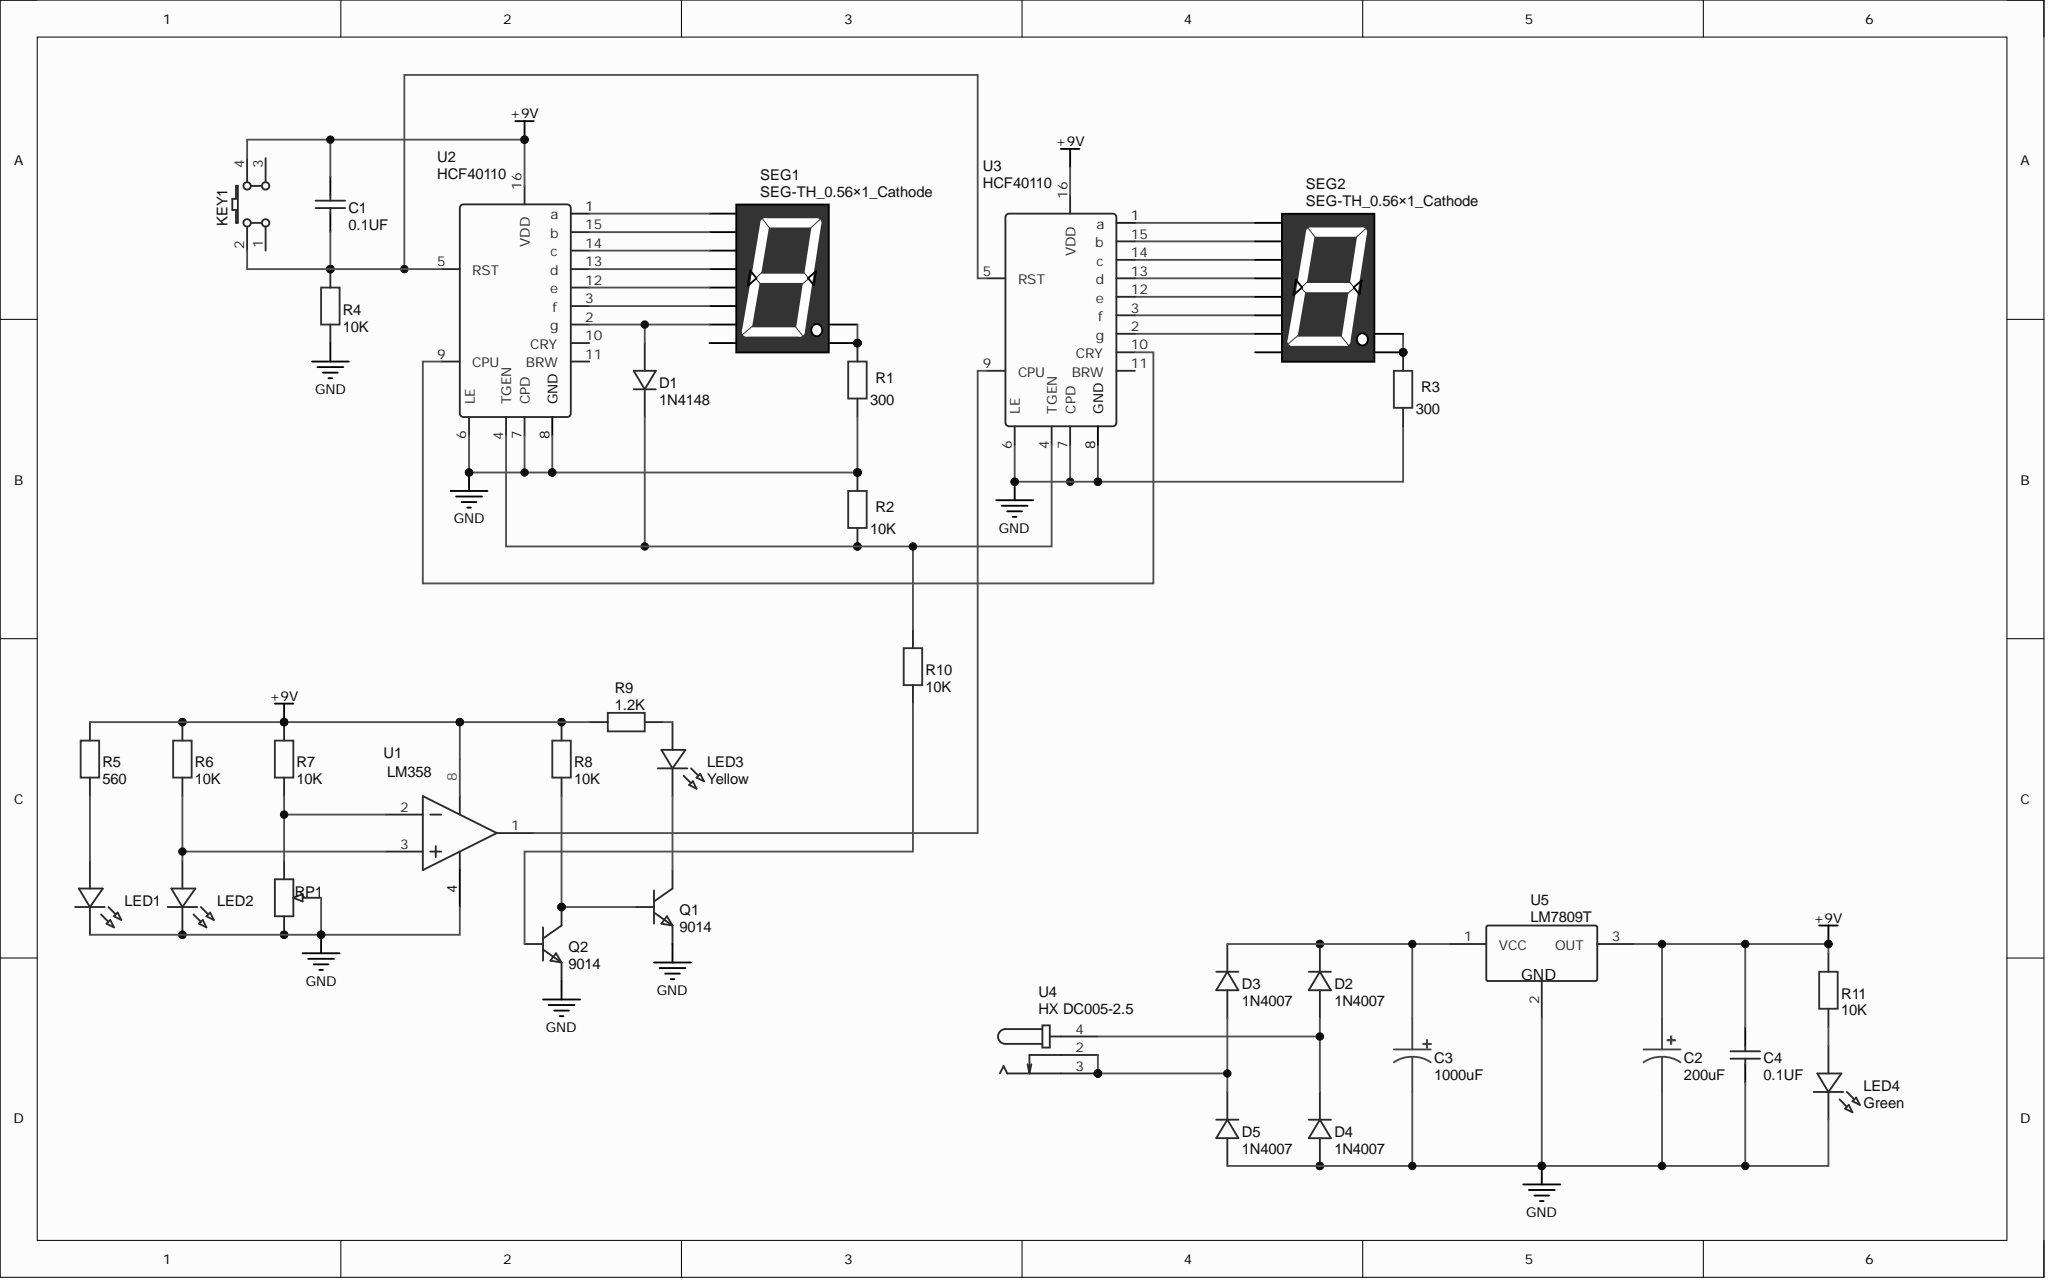Circuit board | Altium Designer | 35 parts | 33 nets
Bill of materials:
Comment,Description,Designator,Footprint,LibRef,Quantity
"0.1UF","","C1, C4","CAP-TH_L5.0-W4.0-P5.00-D1.0","0.1UF","2"
"200uF","","C2","CAP-TH_BD10.0-P5.00-D1.0-FD","200uF","1"
"1000uF","","C3","CAP-TH_BD10.0-P5.00-D1.0-FD","1000uF","1"
"1N4148","","D1","DO-35_BD2.2-L4.0-D0.50_1N4148","1N4148","1"
"1N4007","","D2, D3, D4, D5","DO-41_BD2.4-L4.7-P8.70-D0.9-FD","1N4007","4"
"K4-6×6_TH","","KEY1","KEY-TH_4P-L6.0-W6.0-P4.50-LS6.5","K4-6×6_TH","1"
"LED-TH-5mm_R","","LED1, LED2","LED-TH_BD5.0_RED","LED-TH-5mm_R","2"
"Yellow","","LED3","LED-TH_BD5.0_RED","黄","1"
"Green","","LED4","LED-TH_BD5.0_RED","绿","1"
"9014","","Q1, Q2","TO-92-3_L4.9-W3.7-P2.54-L","9014","2"
"300","","R1, R3","R_AXIAL-0.4","300","2"
"10K","","R2, R4, R6, R7, R8, R10, R11","R_AXIAL-0.4","10K","7"
"560","","R5","R_AXIAL-0.4","560","1"
"1.2K","","R9","R_AXIAL-0.4","1.2K","1"
"R_3386P_EU","","RP1","RES-ADJ-TH_3386P","R_3386P_EU","1"
"SEG-TH_0.56×1_Cathode","","SEG1, SEG2","LED-SEG-TH_10P-L12.6-W19.0-P2.54-S15.24-BL","SEG-TH_0.56×1_Cathode","2"
"LM358","","U1","DIP-8_L8.8-W6.4-P2.54-LS7.6-BL","LM358","1"
"HCF40110","","U2, U3","DIP-16_16P-L20.2-W6.6-P2.54-LS7.6-BL","HCF40110","2"
"HX DC005-2.5","","U4","DC-IN-TH_HX-DC005-2.5","HX DC005-2.5","1"
"LM7809T","","U5","TO-220-3_L10.0-W4.5-P2.54-L","LM7809T","1"
Netlist (Protel format):
[
C1
CAP-TH_L5.0-W4.0-P5.00-D1.0
0.1UF



]
[
C2
CAP-TH_BD10.0-P5.00-D1.0-FD
200uF



]
[
C3
CAP-TH_BD10.0-P5.00-D1.0-FD
1000uF



]
[
C4
CAP-TH_L5.0-W4.0-P5.00-D1.0
0.1UF



]
[
D1
DO-35_BD2.2-L4.0-D0.50_1N4148
1N4148



]
[
D2
DO-41_BD2.4-L4.7-P8.70-D0.9-FD
1N4007



]
[
D3
DO-41_BD2.4-L4.7-P8.70-D0.9-FD
1N4007



]
[
D4
DO-41_BD2.4-L4.7-P8.70-D0.9-FD
1N4007



]
[
D5
DO-41_BD2.4-L4.7-P8.70-D0.9-FD
1N4007



]
[
KEY1
KEY-TH_4P-L6.0-W6.0-P4.50-LS6.5
K4-6×6_TH



]
[
LED1
LED-TH_BD5.0_RED
LED-TH-5mm_R



]
[
LED2
LED-TH_BD5.0_RED
LED-TH-5mm_R



]
[
LED3
LED-TH_BD5.0_RED
Yellow



]
[
LED4
LED-TH_BD5.0_RED
Green



]
[
Q1
TO-92-3_L4.9-W3.7-P2.54-L
9014



]
[
Q2
TO-92-3_L4.9-W3.7-P2.54-L
9014



]
[
R1
R_AXIAL-0.4
300



]
[
R2
R_AXIAL-0.4
10K



]
[
R3
R_AXIAL-0.4
300



]
[
R4
R_AXIAL-0.4
10K



]
[
R5
R_AXIAL-0.4
560



]
[
R6
R_AXIAL-0.4
10K



]
[
R7
R_AXIAL-0.4
10K



]
[
R8
R_AXIAL-0.4
10K



]
[
R9
R_AXIAL-0.4
1.2K



]
[
R10
R_AXIAL-0.4
10K



]
[
R11
R_AXIAL-0.4
10K



]
[
RP1
RES-ADJ-TH_3386P
R_3386P_EU



]
[
SEG1
LED-SEG-TH_10P-L12.6-W19.0-P2.54-S15.24-BL
SEG-TH_0.56×1_Cathode



]
[
SEG2
LED-SEG-TH_10P-L12.6-W19.0-P2.54-S15.24-BL
SEG-TH_0.56×1_Cathode



]
[
U1
DIP-8_L8.8-W6.4-P2.54-LS7.6-BL
LM358



]
[
U2
DIP-16_16P-L20.2-W6.6-P2.54-LS7.6-BL
HCF40110



]
[
U3
DIP-16_16P-L20.2-W6.6-P2.54-LS7.6-BL
HCF40110



]
[
U4
DC-IN-TH_HX-DC005-2.5
HX DC005-2.5



]
[
U5
TO-220-3_L10.0-W4.5-P2.54-L
LM7809T



]
(
NetU2_9
U2-9
U3-10
)
(
NetU1_1
U1-1
U3-9
)
(
NetSEG2_10
SEG2-10
U3-2
)
(
NetSEG2_9
SEG2-9
U3-3
)
(
NetSEG2_7
SEG2-7
U3-1
)
(
NetSEG2_6
SEG2-6
U3-15
)
(
NetSEG2_4
SEG2-4
U3-14
)
(
NetSEG2_2
SEG2-2
U3-13
)
(
NetSEG2_1
SEG2-1
U3-12
)
(
NetSEG1_9
SEG1-9
U2-3
)
(
NetSEG1_7
SEG1-7
U2-1
)
(
NetSEG1_6
SEG1-6
U2-15
)
(
NetSEG1_4
SEG1-4
U2-14
)
(
NetSEG1_2
SEG1-2
U2-13
)
(
NetSEG1_1
SEG1-1
U2-12
)
(
NetR7_1
R7-1
RP1-1
U1-2
)
(
NetR3_2
R3-2
SEG2-3
SEG2-8
)
(
NetR1_2
R1-2
SEG1-3
SEG1-8
)
(
NetQ2_2
Q2-2
R10-1
)
(
NetQ1_2
Q1-2
Q2-3
R8-1
)
(
NetLED4_1
LED4-1
R11-1
)
(
NetLED3_2
LED3-2
Q1-3
)
(
NetLED3_1
LED3-1
R9-1
)
(
NetLED2_1
LED2-1
R6-1
U1-3
)
(
NetLED1_1
LED1-1
R5-1
)
(
NetD3_1
D3-1
D5-2
U4-2
U4-3
)
(
NetD2_1
D2-1
D4-2
U4-4
)
(
NetD1_2
D1-2
R2-1
R10-2
U2-4
U3-4
)
(
NetD1_1
D1-1
SEG1-10
U2-2
)
(
NetC3_1
C3-1
D2-2
D3-2
U5-1
)
(
NetC1_1
C1-1
KEY1-2
R4-2
U2-5
U3-5
)
(
GND
C2-2
C3-2
C4-1
D4-1
D5-1
LED1-2
LED2-2
LED4-2
Q1-1
Q2-1
R1-1
R2-2
R3-1
R4-1
RP1-2
RP1-3
U1-4
U2-6
U2-7
U2-8
U3-6
U3-7
U3-8
U5-2
)
(
+9V
C1-2
C2-1
C4-2
KEY1-4
R5-2
R6-2
R7-2
R8-2
R9-2
R11-2
U1-8
U2-16
U3-16
U5-3
)